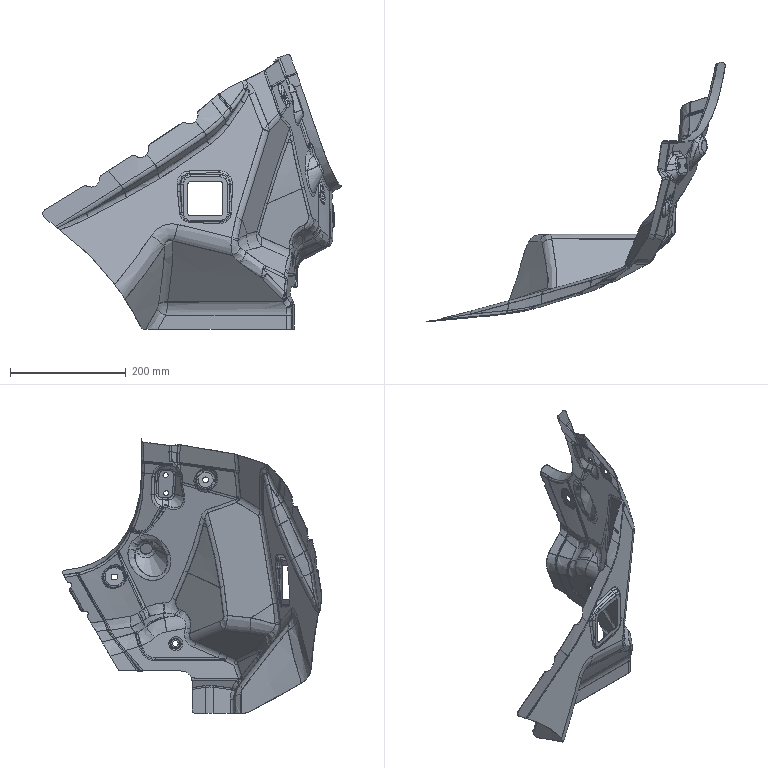Part | STEP file | FNA5401151 | 1 solid | 892 faces | box 516 x 448.464 x 475.039 mm | volume 197748 mm3 | spline 726 | cylinder 93 | plane 49 | other 20 | sphere 4 | commonest cylinder face diameters 10 x10 16 x7 40 x5 2 x4 8 x4 8.4 x4